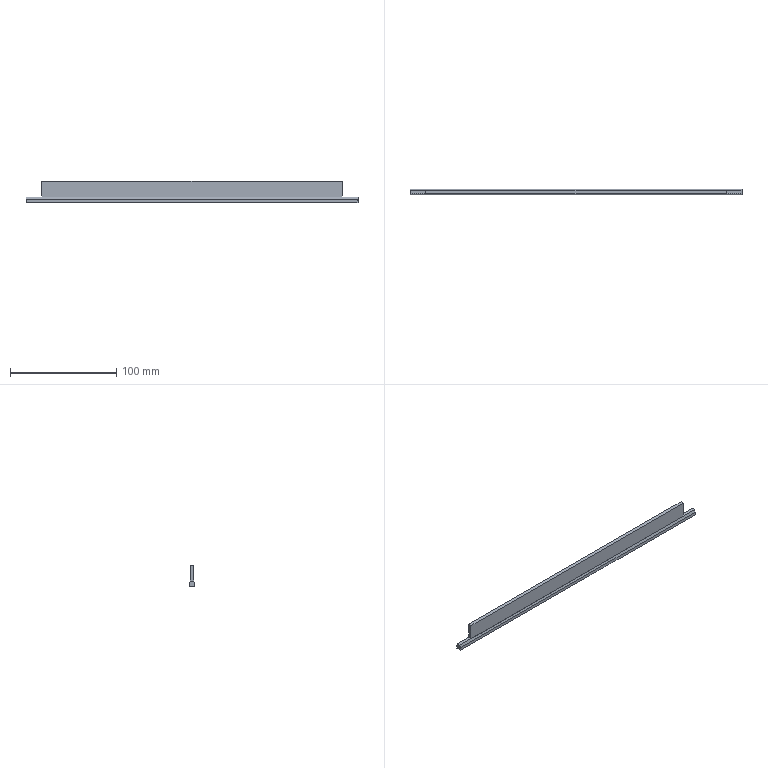Part | SolidWorks | features ICE 2, Extrusion 1 | 1 solid | 13 faces | box 313 x 5 x 20.5 mm | volume 20756 mm3 | plane 13
STEP:
#1=CARTESIAN_POINT('',(-156.5,-1.75,5.5));
#2=VERTEX_POINT('',#1);
#3=CARTESIAN_POINT('',(156.5,-1.75,5.5));
#4=VERTEX_POINT('',#3);
#5=CARTESIAN_POINT('',(-156.5,-1.75,5.5));
#6=DIRECTION('',(1.,0.,0.));
#7=VECTOR('',#6,1000.);
#8=LINE('',#5,#7);
#9=EDGE_CURVE('',#2,#4,#8,.T.);
#10=ORIENTED_EDGE('',*,*,#9,.T.);
#11=CARTESIAN_POINT('',(156.5,1.75,5.5));
#12=VERTEX_POINT('',#11);
#13=CARTESIAN_POINT('',(156.5,2.5,5.5));
#14=DIRECTION('',(0.,1.,0.));
#15=VECTOR('',#14,1000.);
#16=LINE('',#13,#15);
#17=EDGE_CURVE('',#4,#12,#16,.T.);
#18=ORIENTED_EDGE('',*,*,#17,.T.);
#19=CARTESIAN_POINT('',(-156.5,1.75,5.5));
#20=VERTEX_POINT('',#19);
#21=CARTESIAN_POINT('',(-156.5,1.75,5.5));
#22=DIRECTION('',(1.,0.,0.));
#23=VECTOR('',#22,1000.);
#24=LINE('',#21,#23);
#25=EDGE_CURVE('',#20,#12,#24,.T.);
#26=ORIENTED_EDGE('',*,*,#25,.F.);
#27=CARTESIAN_POINT('',(-156.5,2.5,5.5));
#28=DIRECTION('',(0.,-1.,0.));
#29=VECTOR('',#28,1000.);
#30=LINE('',#27,#29);
#31=EDGE_CURVE('',#20,#2,#30,.T.);
#32=ORIENTED_EDGE('',*,*,#31,.T.);
#33=EDGE_LOOP('',(#10,#18,#26,#32));
#34=FACE_OUTER_BOUND('',#33,.T.);
#35=CARTESIAN_POINT('',(141.5,1.5,5.5));
#36=VERTEX_POINT('',#35);
#37=CARTESIAN_POINT('',(-141.5,1.5,5.5));
#38=VERTEX_POINT('',#37);
#39=CARTESIAN_POINT('',(-141.5,1.5,5.5));
#40=DIRECTION('',(-1.,0.,0.));
#41=VECTOR('',#40,1000.);
#42=LINE('',#39,#41);
#43=EDGE_CURVE('',#36,#38,#42,.T.);
#44=ORIENTED_EDGE('',*,*,#43,.F.);
#45=CARTESIAN_POINT('',(141.5,-1.5,5.5));
#46=VERTEX_POINT('',#45);
#47=CARTESIAN_POINT('',(141.5,-1.5,5.5));
#48=DIRECTION('',(0.,1.,0.));
#49=VECTOR('',#48,1000.);
#50=LINE('',#47,#49);
#51=EDGE_CURVE('',#46,#36,#50,.T.);
#52=ORIENTED_EDGE('',*,*,#51,.F.);
#53=CARTESIAN_POINT('',(-141.5,-1.5,5.5));
#54=VERTEX_POINT('',#53);
#55=CARTESIAN_POINT('',(-141.5,-1.5,5.5));
#56=DIRECTION('',(1.,0.,0.));
#57=VECTOR('',#56,1000.);
#58=LINE('',#55,#57);
#59=EDGE_CURVE('',#54,#46,#58,.T.);
#60=ORIENTED_EDGE('',*,*,#59,.F.);
#61=CARTESIAN_POINT('',(-141.5,-1.5,5.5));
#62=DIRECTION('',(0.,-1.,0.));
#63=VECTOR('',#62,1000.);
#64=LINE('',#61,#63);
#65=EDGE_CURVE('',#38,#54,#64,.T.);
#66=ORIENTED_EDGE('',*,*,#65,.F.);
#67=EDGE_LOOP('',(#44,#52,#60,#66));
#68=FACE_BOUND('',#67,.T.);
#69=CARTESIAN_POINT('',(0.,0.,5.5));
#70=DIRECTION('',(0.,0.,1.));
#71=DIRECTION('',(1.,0.,0.));
#72=AXIS2_PLACEMENT_3D('',#69,#70,#71);
#73=PLANE('',#72);
#74=ADVANCED_FACE('',(#34,#68),#73,.T.);
#75=ORIENTED_EDGE('',*,*,#17,.F.);
#76=CARTESIAN_POINT('',(156.5,-2.5,3.));
#77=VERTEX_POINT('',#76);
#78=CARTESIAN_POINT('',(156.5,-2.5,3.));
#79=DIRECTION('',(0.,0.2873,0.9578));
#80=VECTOR('',#79,1000.);
#81=LINE('',#78,#80);
#82=EDGE_CURVE('',#77,#4,#81,.T.);
#83=ORIENTED_EDGE('',*,*,#82,.F.);
#84=CARTESIAN_POINT('',(156.5,-2.5,0.));
#85=VERTEX_POINT('',#84);
#86=CARTESIAN_POINT('',(156.5,-2.5,5.5));
#87=DIRECTION('',(0.,0.,-1.));
#88=VECTOR('',#87,1000.);
#89=LINE('',#86,#88);
#90=EDGE_CURVE('',#77,#85,#89,.T.);
#91=ORIENTED_EDGE('',*,*,#90,.T.);
#92=CARTESIAN_POINT('',(156.5,2.5,0.));
#93=VERTEX_POINT('',#92);
#94=CARTESIAN_POINT('',(156.5,2.5,0.));
#95=DIRECTION('',(0.,1.,0.));
#96=VECTOR('',#95,1000.);
#97=LINE('',#94,#96);
#98=EDGE_CURVE('',#85,#93,#97,.T.);
#99=ORIENTED_EDGE('',*,*,#98,.T.);
#100=CARTESIAN_POINT('',(156.5,2.5,3.));
#101=VERTEX_POINT('',#100);
#102=CARTESIAN_POINT('',(156.5,2.5,5.5));
#103=DIRECTION('',(0.,0.,-1.));
#104=VECTOR('',#103,1000.);
#105=LINE('',#102,#104);
#106=EDGE_CURVE('',#101,#93,#105,.T.);
#107=ORIENTED_EDGE('',*,*,#106,.F.);
#108=CARTESIAN_POINT('',(156.5,2.5,3.));
#109=DIRECTION('',(0.,0.2873,-0.9578));
#110=VECTOR('',#109,1000.);
#111=LINE('',#108,#110);
#112=EDGE_CURVE('',#12,#101,#111,.T.);
#113=ORIENTED_EDGE('',*,*,#112,.F.);
#114=EDGE_LOOP('',(#75,#83,#91,#99,#107,#113));
#115=FACE_OUTER_BOUND('',#114,.T.);
#116=CARTESIAN_POINT('',(156.5,2.5,5.5));
#117=DIRECTION('',(-1.,0.,0.));
#118=DIRECTION('',(0.,0.,1.));
#119=AXIS2_PLACEMENT_3D('',#116,#117,#118);
#120=PLANE('',#119);
#121=ADVANCED_FACE('',(#115),#120,.F.);
#122=CARTESIAN_POINT('',(-156.5,2.5,3.));
#123=VERTEX_POINT('',#122);
#124=CARTESIAN_POINT('',(-156.5,2.5,0.));
#125=VERTEX_POINT('',#124);
#126=CARTESIAN_POINT('',(-156.5,2.5,5.5));
#127=DIRECTION('',(0.,0.,-1.));
#128=VECTOR('',#127,1000.);
#129=LINE('',#126,#128);
#130=EDGE_CURVE('',#123,#125,#129,.T.);
#131=ORIENTED_EDGE('',*,*,#130,.F.);
#132=CARTESIAN_POINT('',(-156.5,2.5,3.));
#133=DIRECTION('',(1.,0.,0.));
#134=VECTOR('',#133,1000.);
#135=LINE('',#132,#134);
#136=EDGE_CURVE('',#123,#101,#135,.T.);
#137=ORIENTED_EDGE('',*,*,#136,.T.);
#138=ORIENTED_EDGE('',*,*,#106,.T.);
#139=CARTESIAN_POINT('',(-156.5,2.5,0.));
#140=DIRECTION('',(-1.,0.,0.));
#141=VECTOR('',#140,1000.);
#142=LINE('',#139,#141);
#143=EDGE_CURVE('',#93,#125,#142,.T.);
#144=ORIENTED_EDGE('',*,*,#143,.T.);
#145=EDGE_LOOP('',(#131,#137,#138,#144));
#146=FACE_OUTER_BOUND('',#145,.T.);
#147=CARTESIAN_POINT('',(-156.5,2.5,5.5));
#148=DIRECTION('',(0.,-1.,0.));
#149=DIRECTION('',(0.,0.,-1.));
#150=AXIS2_PLACEMENT_3D('',#147,#148,#149);
#151=PLANE('',#150);
#152=ADVANCED_FACE('',(#146),#151,.F.);
#153=CARTESIAN_POINT('',(-156.5,-2.5,3.));
#154=VERTEX_POINT('',#153);
#155=CARTESIAN_POINT('',(-156.5,-2.5,0.));
#156=VERTEX_POINT('',#155);
#157=CARTESIAN_POINT('',(-156.5,-2.5,5.5));
#158=DIRECTION('',(0.,0.,-1.));
#159=VECTOR('',#158,1000.);
#160=LINE('',#157,#159);
#161=EDGE_CURVE('',#154,#156,#160,.T.);
#162=ORIENTED_EDGE('',*,*,#161,.F.);
#163=CARTESIAN_POINT('',(-156.5,-2.5,3.));
#164=DIRECTION('',(0.,0.2873,0.9578));
#165=VECTOR('',#164,1000.);
#166=LINE('',#163,#165);
#167=EDGE_CURVE('',#154,#2,#166,.T.);
#168=ORIENTED_EDGE('',*,*,#167,.T.);
#169=ORIENTED_EDGE('',*,*,#31,.F.);
#170=CARTESIAN_POINT('',(-156.5,2.5,3.));
#171=DIRECTION('',(0.,0.2873,-0.9578));
#172=VECTOR('',#171,1000.);
#173=LINE('',#170,#172);
#174=EDGE_CURVE('',#20,#123,#173,.T.);
#175=ORIENTED_EDGE('',*,*,#174,.T.);
#176=ORIENTED_EDGE('',*,*,#130,.T.);
#177=CARTESIAN_POINT('',(-156.5,2.5,0.));
#178=DIRECTION('',(0.,-1.,0.));
#179=VECTOR('',#178,1000.);
#180=LINE('',#177,#179);
#181=EDGE_CURVE('',#125,#156,#180,.T.);
#182=ORIENTED_EDGE('',*,*,#181,.T.);
#183=EDGE_LOOP('',(#162,#168,#169,#175,#176,#182));
#184=FACE_OUTER_BOUND('',#183,.T.);
#185=CARTESIAN_POINT('',(-156.5,2.5,5.5));
#186=DIRECTION('',(1.,0.,0.));
#187=DIRECTION('',(0.,0.,-1.));
#188=AXIS2_PLACEMENT_3D('',#185,#186,#187);
#189=PLANE('',#188);
#190=ADVANCED_FACE('',(#184),#189,.F.);
#191=ORIENTED_EDGE('',*,*,#90,.F.);
#192=CARTESIAN_POINT('',(-156.5,-2.5,3.));
#193=DIRECTION('',(1.,0.,0.));
#194=VECTOR('',#193,1000.);
#195=LINE('',#192,#194);
#196=EDGE_CURVE('',#154,#77,#195,.T.);
#197=ORIENTED_EDGE('',*,*,#196,.F.);
#198=ORIENTED_EDGE('',*,*,#161,.T.);
#199=CARTESIAN_POINT('',(-156.5,-2.5,0.));
#200=DIRECTION('',(1.,0.,0.));
#201=VECTOR('',#200,1000.);
#202=LINE('',#199,#201);
#203=EDGE_CURVE('',#156,#85,#202,.T.);
#204=ORIENTED_EDGE('',*,*,#203,.T.);
#205=EDGE_LOOP('',(#191,#197,#198,#204));
#206=FACE_OUTER_BOUND('',#205,.T.);
#207=CARTESIAN_POINT('',(-156.5,-2.5,5.5));
#208=DIRECTION('',(0.,1.,0.));
#209=DIRECTION('',(0.,0.,1.));
#210=AXIS2_PLACEMENT_3D('',#207,#208,#209);
#211=PLANE('',#210);
#212=ADVANCED_FACE('',(#206),#211,.F.);
#213=ORIENTED_EDGE('',*,*,#98,.F.);
#214=ORIENTED_EDGE('',*,*,#203,.F.);
#215=ORIENTED_EDGE('',*,*,#181,.F.);
#216=ORIENTED_EDGE('',*,*,#143,.F.);
#217=EDGE_LOOP('',(#213,#214,#215,#216));
#218=FACE_OUTER_BOUND('',#217,.T.);
#219=CARTESIAN_POINT('',(0.,0.,0.));
#220=DIRECTION('',(0.,0.,1.));
#221=DIRECTION('',(1.,0.,0.));
#222=AXIS2_PLACEMENT_3D('',#219,#220,#221);
#223=PLANE('',#222);
#224=ADVANCED_FACE('',(#218),#223,.F.);
#225=ORIENTED_EDGE('',*,*,#112,.T.);
#226=ORIENTED_EDGE('',*,*,#136,.F.);
#227=ORIENTED_EDGE('',*,*,#174,.F.);
#228=ORIENTED_EDGE('',*,*,#25,.T.);
#229=EDGE_LOOP('',(#225,#226,#227,#228));
#230=FACE_OUTER_BOUND('',#229,.T.);
#231=CARTESIAN_POINT('',(-156.5,2.5,3.));
#232=DIRECTION('',(0.,-0.9578,-0.2873));
#233=DIRECTION('',(0.,0.2873,-0.9578));
#234=AXIS2_PLACEMENT_3D('',#231,#232,#233);
#235=PLANE('',#234);
#236=ADVANCED_FACE('',(#230),#235,.F.);
#237=ORIENTED_EDGE('',*,*,#82,.T.);
#238=ORIENTED_EDGE('',*,*,#9,.F.);
#239=ORIENTED_EDGE('',*,*,#167,.F.);
#240=ORIENTED_EDGE('',*,*,#196,.T.);
#241=EDGE_LOOP('',(#237,#238,#239,#240));
#242=FACE_OUTER_BOUND('',#241,.T.);
#243=CARTESIAN_POINT('',(-156.5,-2.5,3.));
#244=DIRECTION('',(0.,0.9578,-0.2873));
#245=DIRECTION('',(0.,0.2873,0.9578));
#246=AXIS2_PLACEMENT_3D('',#243,#244,#245);
#247=PLANE('',#246);
#248=ADVANCED_FACE('',(#242),#247,.F.);
#249=ORIENTED_EDGE('',*,*,#51,.T.);
#250=CARTESIAN_POINT('',(141.5,1.5,20.5));
#251=VERTEX_POINT('',#250);
#252=CARTESIAN_POINT('',(141.5,1.5,20.5));
#253=DIRECTION('',(0.,0.,-1.));
#254=VECTOR('',#253,1000.);
#255=LINE('',#252,#254);
#256=EDGE_CURVE('',#251,#36,#255,.T.);
#257=ORIENTED_EDGE('',*,*,#256,.F.);
#258=CARTESIAN_POINT('',(141.5,-1.5,20.5));
#259=VERTEX_POINT('',#258);
#260=CARTESIAN_POINT('',(141.5,-1.5,20.5));
#261=DIRECTION('',(0.,1.,0.));
#262=VECTOR('',#261,1000.);
#263=LINE('',#260,#262);
#264=EDGE_CURVE('',#259,#251,#263,.T.);
#265=ORIENTED_EDGE('',*,*,#264,.F.);
#266=CARTESIAN_POINT('',(141.5,-1.5,20.5));
#267=DIRECTION('',(0.,0.,-1.));
#268=VECTOR('',#267,1000.);
#269=LINE('',#266,#268);
#270=EDGE_CURVE('',#259,#46,#269,.T.);
#271=ORIENTED_EDGE('',*,*,#270,.T.);
#272=EDGE_LOOP('',(#249,#257,#265,#271));
#273=FACE_OUTER_BOUND('',#272,.T.);
#274=CARTESIAN_POINT('',(141.5,-1.5,20.5));
#275=DIRECTION('',(-1.,0.,0.));
#276=DIRECTION('',(0.,0.,1.));
#277=AXIS2_PLACEMENT_3D('',#274,#275,#276);
#278=PLANE('',#277);
#279=ADVANCED_FACE('',(#273),#278,.F.);
#280=ORIENTED_EDGE('',*,*,#43,.T.);
#281=CARTESIAN_POINT('',(-141.5,1.5,20.5));
#282=VERTEX_POINT('',#281);
#283=CARTESIAN_POINT('',(-141.5,1.5,20.5));
#284=DIRECTION('',(0.,0.,-1.));
#285=VECTOR('',#284,1000.);
#286=LINE('',#283,#285);
#287=EDGE_CURVE('',#282,#38,#286,.T.);
#288=ORIENTED_EDGE('',*,*,#287,.F.);
#289=CARTESIAN_POINT('',(-141.5,1.5,20.5));
#290=DIRECTION('',(-1.,0.,0.));
#291=VECTOR('',#290,1000.);
#292=LINE('',#289,#291);
#293=EDGE_CURVE('',#251,#282,#292,.T.);
#294=ORIENTED_EDGE('',*,*,#293,.F.);
#295=ORIENTED_EDGE('',*,*,#256,.T.);
#296=EDGE_LOOP('',(#280,#288,#294,#295));
#297=FACE_OUTER_BOUND('',#296,.T.);
#298=CARTESIAN_POINT('',(-141.5,1.5,20.5));
#299=DIRECTION('',(0.,-1.,0.));
#300=DIRECTION('',(0.,0.,-1.));
#301=AXIS2_PLACEMENT_3D('',#298,#299,#300);
#302=PLANE('',#301);
#303=ADVANCED_FACE('',(#297),#302,.F.);
#304=ORIENTED_EDGE('',*,*,#65,.T.);
#305=CARTESIAN_POINT('',(-141.5,-1.5,20.5));
#306=VERTEX_POINT('',#305);
#307=CARTESIAN_POINT('',(-141.5,-1.5,20.5));
#308=DIRECTION('',(0.,0.,-1.));
#309=VECTOR('',#308,1000.);
#310=LINE('',#307,#309);
#311=EDGE_CURVE('',#306,#54,#310,.T.);
#312=ORIENTED_EDGE('',*,*,#311,.F.);
#313=CARTESIAN_POINT('',(-141.5,-1.5,20.5));
#314=DIRECTION('',(0.,-1.,0.));
#315=VECTOR('',#314,1000.);
#316=LINE('',#313,#315);
#317=EDGE_CURVE('',#282,#306,#316,.T.);
#318=ORIENTED_EDGE('',*,*,#317,.F.);
#319=ORIENTED_EDGE('',*,*,#287,.T.);
#320=EDGE_LOOP('',(#304,#312,#318,#319));
#321=FACE_OUTER_BOUND('',#320,.T.);
#322=CARTESIAN_POINT('',(-141.5,-1.5,20.5));
#323=DIRECTION('',(1.,0.,0.));
#324=DIRECTION('',(0.,0.,-1.));
#325=AXIS2_PLACEMENT_3D('',#322,#323,#324);
#326=PLANE('',#325);
#327=ADVANCED_FACE('',(#321),#326,.F.);
#328=ORIENTED_EDGE('',*,*,#59,.T.);
#329=ORIENTED_EDGE('',*,*,#270,.F.);
#330=CARTESIAN_POINT('',(-141.5,-1.5,20.5));
#331=DIRECTION('',(1.,0.,0.));
#332=VECTOR('',#331,1000.);
#333=LINE('',#330,#332);
#334=EDGE_CURVE('',#306,#259,#333,.T.);
#335=ORIENTED_EDGE('',*,*,#334,.F.);
#336=ORIENTED_EDGE('',*,*,#311,.T.);
#337=EDGE_LOOP('',(#328,#329,#335,#336));
#338=FACE_OUTER_BOUND('',#337,.T.);
#339=CARTESIAN_POINT('',(-141.5,-1.5,20.5));
#340=DIRECTION('',(0.,1.,0.));
#341=DIRECTION('',(0.,0.,1.));
#342=AXIS2_PLACEMENT_3D('',#339,#340,#341);
#343=PLANE('',#342);
#344=ADVANCED_FACE('',(#338),#343,.F.);
#345=ORIENTED_EDGE('',*,*,#264,.T.);
#346=ORIENTED_EDGE('',*,*,#293,.T.);
#347=ORIENTED_EDGE('',*,*,#317,.T.);
#348=ORIENTED_EDGE('',*,*,#334,.T.);
#349=EDGE_LOOP('',(#345,#346,#347,#348));
#350=FACE_OUTER_BOUND('',#349,.T.);
#351=CARTESIAN_POINT('',(0.,0.,20.5));
#352=DIRECTION('',(0.,0.,-1.));
#353=DIRECTION('',(-1.,0.,0.));
#354=AXIS2_PLACEMENT_3D('',#351,#352,#353);
#355=PLANE('',#354);
#356=ADVANCED_FACE('',(#350),#355,.F.);
#357=CLOSED_SHELL('',(#74,#121,#152,#190,#212,#224,#236,#248,#279,#303,#327,#344,#356));
#358=MANIFOLD_SOLID_BREP('',#357);
#359=CARTESIAN_POINT('',(0.,0.,0.));
#360=DIRECTION('',(0.,0.,1.));
#361=DIRECTION('',(1.,0.,0.));
#362=AXIS2_PLACEMENT_3D('',#359,#360,#361);
#363=(LENGTH_UNIT()NAMED_UNIT(*)SI_UNIT(.MILLI.,.METRE.));
#364=UNCERTAINTY_MEASURE_WITH_UNIT(LENGTH_MEASURE(0.00001),#363,'','');
#365=(NAMED_UNIT(*)PLANE_ANGLE_UNIT()SI_UNIT($,.RADIAN.));
#366=(NAMED_UNIT(*)SI_UNIT($,.STERADIAN.)SOLID_ANGLE_UNIT());
#367=(GEOMETRIC_REPRESENTATION_CONTEXT(3)GLOBAL_UNCERTAINTY_ASSIGNED_CONTEXT((#364))GLOBAL_UNIT_ASSIGNED_CONTEXT((#363,#365,#366))REPRESENTATION_CONTEXT('',''));
#368=ADVANCED_BREP_SHAPE_REPRESENTATION('',(#358,#362),#367);